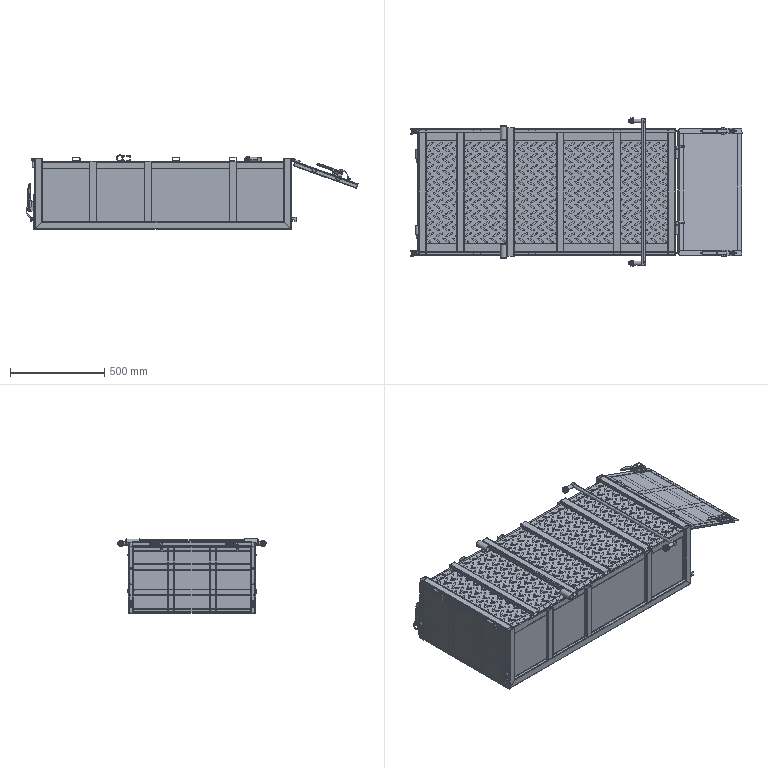Part | SolidWorks | 72 solids | 5232 faces | volume 8277423 mm3 | spline 2232 | plane 1782 | cylinder 550 | sphere 432 | torus 188 | cone 48 | commonest cylinder face diameters 6 x168 2 x68 28.8 x32 8 x28 4 x24 10 x20